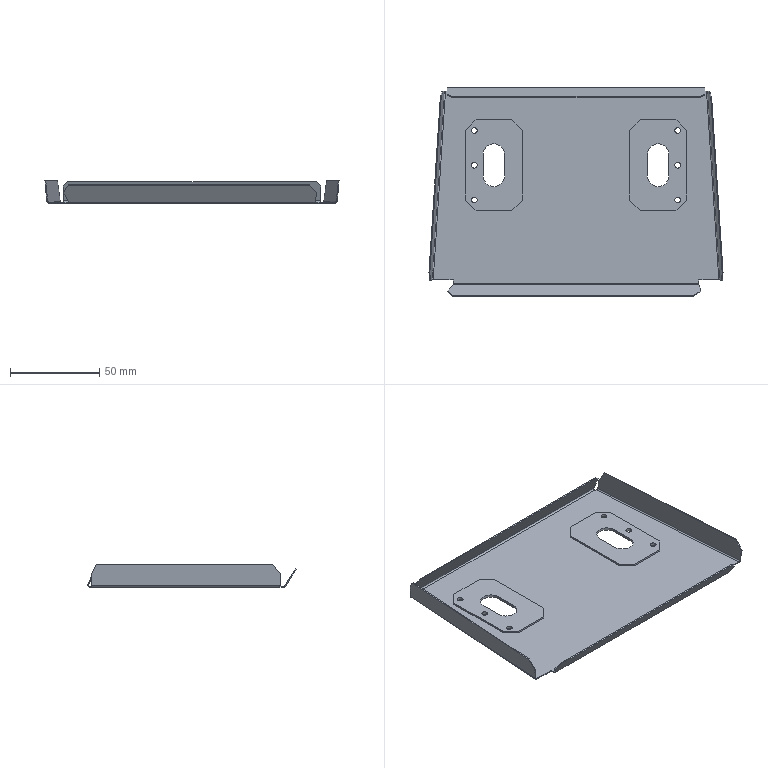Part | SolidWorks | features BaseBody 1 | 1 solid | 89 faces | box 164.763 x 116.676 x 12.729 mm | volume 13737 mm3 | plane 59 | cylinder 24 | spline 6 | commonest cylinder face diameters 3.2 x12 1.5 x4 2.5 x4 12 x4